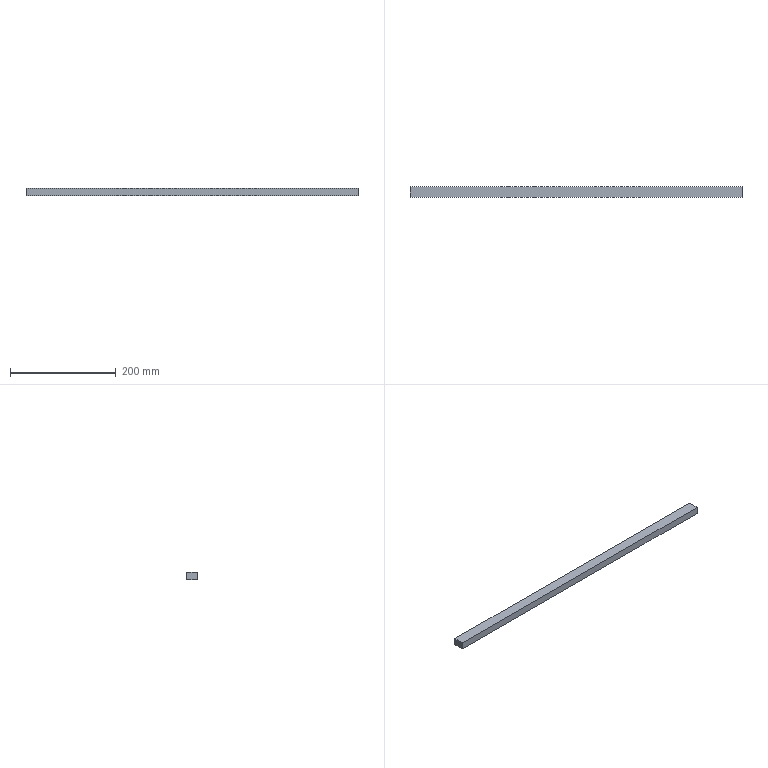Part | STEP file | Cylinder hanging plate | 1 solid | 6 faces | box 627.6 x 20 x 14 mm | volume 175728 mm3 | plane 6
STEP:
#1=CARTESIAN_POINT('',(0.,0.,0.));
#2=DIRECTION('',(0.,0.,1.));
#3=DIRECTION('',(1.,0.,0.));
#4=AXIS2_PLACEMENT_3D('',#1,#2,#3);
#5=CARTESIAN_POINT('',(313.8,-10.,0.));
#6=VERTEX_POINT('',#5);
#7=CARTESIAN_POINT('',(313.8,10.,0.));
#8=VERTEX_POINT('',#7);
#9=CARTESIAN_POINT('',(313.8,10.,0.));
#10=DIRECTION('',(0.,1.,0.));
#11=VECTOR('',#10,1.);
#12=LINE('',#9,#11);
#13=CARTESIAN_POINT('',(313.8,10.,14.));
#14=DIRECTION('',(-1.,0.,0.));
#15=DIRECTION('',(0.,0.,1.));
#16=AXIS2_PLACEMENT_3D('',#13,#14,#15);
#17=PLANE('',#16);
#18=CARTESIAN_POINT('',(-14.,0.));
#19=DIRECTION('',(0.,1.));
#20=VECTOR('',#19,1.);
#21=LINE('',#18,#20);
#22=(GEOMETRIC_REPRESENTATION_CONTEXT(2)PARAMETRIC_REPRESENTATION_CONTEXT()REPRESENTATION_CONTEXT('',''));
#23=DEFINITIONAL_REPRESENTATION('',(#21),#22);
#24=PCURVE('',#17,#23);
#25=CARTESIAN_POINT('',(313.8,-10.,0.));
#26=DIRECTION('',(0.,0.,1.));
#27=DIRECTION('',(1.,0.,0.));
#28=AXIS2_PLACEMENT_3D('',#25,#26,#27);
#29=PLANE('',#28);
#30=CARTESIAN_POINT('',(0.,20.));
#31=DIRECTION('',(0.,1.));
#32=VECTOR('',#31,1.);
#33=LINE('',#30,#32);
#34=(GEOMETRIC_REPRESENTATION_CONTEXT(2)PARAMETRIC_REPRESENTATION_CONTEXT()REPRESENTATION_CONTEXT('',''));
#35=DEFINITIONAL_REPRESENTATION('',(#33),#34);
#36=PCURVE('',#29,#35);
#37=SURFACE_CURVE('',#12,(#24,#36),.PCURVE_S1.);
#38=EDGE_CURVE('',#6,#8,#37,.T.);
#39=ORIENTED_EDGE('',*,*,#38,.T.);
#40=CARTESIAN_POINT('',(313.8,10.,14.));
#41=VERTEX_POINT('',#40);
#42=CARTESIAN_POINT('',(313.8,10.,14.));
#43=DIRECTION('',(0.,0.,-1.));
#44=VECTOR('',#43,1.);
#45=LINE('',#42,#44);
#46=CARTESIAN_POINT('',(0.,0.));
#47=DIRECTION('',(-1.,0.));
#48=VECTOR('',#47,1.);
#49=LINE('',#46,#48);
#50=(GEOMETRIC_REPRESENTATION_CONTEXT(2)PARAMETRIC_REPRESENTATION_CONTEXT()REPRESENTATION_CONTEXT('',''));
#51=DEFINITIONAL_REPRESENTATION('',(#49),#50);
#52=PCURVE('',#17,#51);
#53=CARTESIAN_POINT('',(-313.8,10.,14.));
#54=DIRECTION('',(0.,-1.,0.));
#55=DIRECTION('',(0.,0.,-1.));
#56=AXIS2_PLACEMENT_3D('',#53,#54,#55);
#57=PLANE('',#56);
#58=CARTESIAN_POINT('',(0.,627.6));
#59=DIRECTION('',(1.,0.));
#60=VECTOR('',#59,1.);
#61=LINE('',#58,#60);
#62=(GEOMETRIC_REPRESENTATION_CONTEXT(2)PARAMETRIC_REPRESENTATION_CONTEXT()REPRESENTATION_CONTEXT('',''));
#63=DEFINITIONAL_REPRESENTATION('',(#61),#62);
#64=PCURVE('',#57,#63);
#65=SURFACE_CURVE('',#45,(#52,#64),.PCURVE_S1.);
#66=EDGE_CURVE('',#41,#8,#65,.T.);
#67=ORIENTED_EDGE('',*,*,#66,.F.);
#68=CARTESIAN_POINT('',(313.8,-10.,14.));
#69=VERTEX_POINT('',#68);
#70=CARTESIAN_POINT('',(313.8,10.,14.));
#71=DIRECTION('',(0.,1.,0.));
#72=VECTOR('',#71,1.);
#73=LINE('',#70,#72);
#74=CARTESIAN_POINT('',(0.,0.));
#75=DIRECTION('',(0.,1.));
#76=VECTOR('',#75,1.);
#77=LINE('',#74,#76);
#78=(GEOMETRIC_REPRESENTATION_CONTEXT(2)PARAMETRIC_REPRESENTATION_CONTEXT()REPRESENTATION_CONTEXT('',''));
#79=DEFINITIONAL_REPRESENTATION('',(#77),#78);
#80=PCURVE('',#17,#79);
#81=CARTESIAN_POINT('',(313.8,-10.,14.));
#82=DIRECTION('',(0.,0.,1.));
#83=DIRECTION('',(1.,0.,0.));
#84=AXIS2_PLACEMENT_3D('',#81,#82,#83);
#85=PLANE('',#84);
#86=CARTESIAN_POINT('',(0.,20.));
#87=DIRECTION('',(0.,1.));
#88=VECTOR('',#87,1.);
#89=LINE('',#86,#88);
#90=(GEOMETRIC_REPRESENTATION_CONTEXT(2)PARAMETRIC_REPRESENTATION_CONTEXT()REPRESENTATION_CONTEXT('',''));
#91=DEFINITIONAL_REPRESENTATION('',(#89),#90);
#92=PCURVE('',#85,#91);
#93=SURFACE_CURVE('',#73,(#80,#92),.PCURVE_S1.);
#94=EDGE_CURVE('',#69,#41,#93,.T.);
#95=ORIENTED_EDGE('',*,*,#94,.F.);
#96=CARTESIAN_POINT('',(313.8,-10.,14.));
#97=DIRECTION('',(0.,0.,-1.));
#98=VECTOR('',#97,1.);
#99=LINE('',#96,#98);
#100=CARTESIAN_POINT('',(0.,-20.));
#101=DIRECTION('',(-1.,0.));
#102=VECTOR('',#101,1.);
#103=LINE('',#100,#102);
#104=(GEOMETRIC_REPRESENTATION_CONTEXT(2)PARAMETRIC_REPRESENTATION_CONTEXT()REPRESENTATION_CONTEXT('',''));
#105=DEFINITIONAL_REPRESENTATION('',(#103),#104);
#106=PCURVE('',#17,#105);
#107=CARTESIAN_POINT('',(-313.8,-10.,14.));
#108=DIRECTION('',(0.,1.,0.));
#109=DIRECTION('',(0.,0.,1.));
#110=AXIS2_PLACEMENT_3D('',#107,#108,#109);
#111=PLANE('',#110);
#112=CARTESIAN_POINT('',(0.,627.6));
#113=DIRECTION('',(-1.,0.));
#114=VECTOR('',#113,1.);
#115=LINE('',#112,#114);
#116=(GEOMETRIC_REPRESENTATION_CONTEXT(2)PARAMETRIC_REPRESENTATION_CONTEXT()REPRESENTATION_CONTEXT('',''));
#117=DEFINITIONAL_REPRESENTATION('',(#115),#116);
#118=PCURVE('',#111,#117);
#119=SURFACE_CURVE('',#99,(#106,#118),.PCURVE_S1.);
#120=EDGE_CURVE('',#69,#6,#119,.T.);
#121=ORIENTED_EDGE('',*,*,#120,.T.);
#122=EDGE_LOOP('',(#39,#67,#95,#121));
#123=FACE_BOUND('',#122,.T.);
#124=ADVANCED_FACE('',(#123),#17,.F.);
#125=CARTESIAN_POINT('',(-313.8,10.,0.));
#126=VERTEX_POINT('',#125);
#127=CARTESIAN_POINT('',(-313.8,10.,0.));
#128=DIRECTION('',(-1.,0.,0.));
#129=VECTOR('',#128,1.);
#130=LINE('',#127,#129);
#131=CARTESIAN_POINT('',(14.,0.));
#132=DIRECTION('',(0.,-1.));
#133=VECTOR('',#132,1.);
#134=LINE('',#131,#133);
#135=(GEOMETRIC_REPRESENTATION_CONTEXT(2)PARAMETRIC_REPRESENTATION_CONTEXT()REPRESENTATION_CONTEXT('',''));
#136=DEFINITIONAL_REPRESENTATION('',(#134),#135);
#137=PCURVE('',#57,#136);
#138=CARTESIAN_POINT('',(-627.6,20.));
#139=DIRECTION('',(-1.,0.));
#140=VECTOR('',#139,1.);
#141=LINE('',#138,#140);
#142=(GEOMETRIC_REPRESENTATION_CONTEXT(2)PARAMETRIC_REPRESENTATION_CONTEXT()REPRESENTATION_CONTEXT('',''));
#143=DEFINITIONAL_REPRESENTATION('',(#141),#142);
#144=PCURVE('',#29,#143);
#145=SURFACE_CURVE('',#130,(#137,#144),.PCURVE_S1.);
#146=EDGE_CURVE('',#8,#126,#145,.T.);
#147=ORIENTED_EDGE('',*,*,#146,.T.);
#148=CARTESIAN_POINT('',(-313.8,10.,14.));
#149=VERTEX_POINT('',#148);
#150=CARTESIAN_POINT('',(-313.8,10.,14.));
#151=DIRECTION('',(0.,0.,-1.));
#152=VECTOR('',#151,1.);
#153=LINE('',#150,#152);
#154=CARTESIAN_POINT('',(0.,0.));
#155=DIRECTION('',(1.,0.));
#156=VECTOR('',#155,1.);
#157=LINE('',#154,#156);
#158=(GEOMETRIC_REPRESENTATION_CONTEXT(2)PARAMETRIC_REPRESENTATION_CONTEXT()REPRESENTATION_CONTEXT('',''));
#159=DEFINITIONAL_REPRESENTATION('',(#157),#158);
#160=PCURVE('',#57,#159);
#161=CARTESIAN_POINT('',(-313.8,10.,14.));
#162=DIRECTION('',(1.,0.,0.));
#163=DIRECTION('',(0.,0.,-1.));
#164=AXIS2_PLACEMENT_3D('',#161,#162,#163);
#165=PLANE('',#164);
#166=CARTESIAN_POINT('',(0.,0.));
#167=DIRECTION('',(1.,0.));
#168=VECTOR('',#167,1.);
#169=LINE('',#166,#168);
#170=(GEOMETRIC_REPRESENTATION_CONTEXT(2)PARAMETRIC_REPRESENTATION_CONTEXT()REPRESENTATION_CONTEXT('',''));
#171=DEFINITIONAL_REPRESENTATION('',(#169),#170);
#172=PCURVE('',#165,#171);
#173=SURFACE_CURVE('',#153,(#160,#172),.PCURVE_S1.);
#174=EDGE_CURVE('',#149,#126,#173,.T.);
#175=ORIENTED_EDGE('',*,*,#174,.F.);
#176=CARTESIAN_POINT('',(-313.8,10.,14.));
#177=DIRECTION('',(-1.,0.,0.));
#178=VECTOR('',#177,1.);
#179=LINE('',#176,#178);
#180=CARTESIAN_POINT('',(0.,0.));
#181=DIRECTION('',(0.,-1.));
#182=VECTOR('',#181,1.);
#183=LINE('',#180,#182);
#184=(GEOMETRIC_REPRESENTATION_CONTEXT(2)PARAMETRIC_REPRESENTATION_CONTEXT()REPRESENTATION_CONTEXT('',''));
#185=DEFINITIONAL_REPRESENTATION('',(#183),#184);
#186=PCURVE('',#57,#185);
#187=CARTESIAN_POINT('',(-627.6,20.));
#188=DIRECTION('',(-1.,0.));
#189=VECTOR('',#188,1.);
#190=LINE('',#187,#189);
#191=(GEOMETRIC_REPRESENTATION_CONTEXT(2)PARAMETRIC_REPRESENTATION_CONTEXT()REPRESENTATION_CONTEXT('',''));
#192=DEFINITIONAL_REPRESENTATION('',(#190),#191);
#193=PCURVE('',#85,#192);
#194=SURFACE_CURVE('',#179,(#186,#193),.PCURVE_S1.);
#195=EDGE_CURVE('',#41,#149,#194,.T.);
#196=ORIENTED_EDGE('',*,*,#195,.F.);
#197=ORIENTED_EDGE('',*,*,#66,.T.);
#198=EDGE_LOOP('',(#147,#175,#196,#197));
#199=FACE_BOUND('',#198,.T.);
#200=ADVANCED_FACE('',(#199),#57,.F.);
#201=CARTESIAN_POINT('',(-313.8,-10.,0.));
#202=VERTEX_POINT('',#201);
#203=CARTESIAN_POINT('',(-313.8,10.,0.));
#204=DIRECTION('',(0.,-1.,0.));
#205=VECTOR('',#204,1.);
#206=LINE('',#203,#205);
#207=CARTESIAN_POINT('',(14.,0.));
#208=DIRECTION('',(0.,-1.));
#209=VECTOR('',#208,1.);
#210=LINE('',#207,#209);
#211=(GEOMETRIC_REPRESENTATION_CONTEXT(2)PARAMETRIC_REPRESENTATION_CONTEXT()REPRESENTATION_CONTEXT('',''));
#212=DEFINITIONAL_REPRESENTATION('',(#210),#211);
#213=PCURVE('',#165,#212);
#214=CARTESIAN_POINT('',(-627.6,20.));
#215=DIRECTION('',(0.,-1.));
#216=VECTOR('',#215,1.);
#217=LINE('',#214,#216);
#218=(GEOMETRIC_REPRESENTATION_CONTEXT(2)PARAMETRIC_REPRESENTATION_CONTEXT()REPRESENTATION_CONTEXT('',''));
#219=DEFINITIONAL_REPRESENTATION('',(#217),#218);
#220=PCURVE('',#29,#219);
#221=SURFACE_CURVE('',#206,(#213,#220),.PCURVE_S1.);
#222=EDGE_CURVE('',#126,#202,#221,.T.);
#223=ORIENTED_EDGE('',*,*,#222,.T.);
#224=CARTESIAN_POINT('',(-313.8,-10.,14.));
#225=VERTEX_POINT('',#224);
#226=CARTESIAN_POINT('',(-313.8,-10.,14.));
#227=DIRECTION('',(0.,0.,-1.));
#228=VECTOR('',#227,1.);
#229=LINE('',#226,#228);
#230=CARTESIAN_POINT('',(0.,-20.));
#231=DIRECTION('',(1.,0.));
#232=VECTOR('',#231,1.);
#233=LINE('',#230,#232);
#234=(GEOMETRIC_REPRESENTATION_CONTEXT(2)PARAMETRIC_REPRESENTATION_CONTEXT()REPRESENTATION_CONTEXT('',''));
#235=DEFINITIONAL_REPRESENTATION('',(#233),#234);
#236=PCURVE('',#165,#235);
#237=CARTESIAN_POINT('',(0.,0.));
#238=DIRECTION('',(-1.,0.));
#239=VECTOR('',#238,1.);
#240=LINE('',#237,#239);
#241=(GEOMETRIC_REPRESENTATION_CONTEXT(2)PARAMETRIC_REPRESENTATION_CONTEXT()REPRESENTATION_CONTEXT('',''));
#242=DEFINITIONAL_REPRESENTATION('',(#240),#241);
#243=PCURVE('',#111,#242);
#244=SURFACE_CURVE('',#229,(#236,#243),.PCURVE_S1.);
#245=EDGE_CURVE('',#225,#202,#244,.T.);
#246=ORIENTED_EDGE('',*,*,#245,.F.);
#247=CARTESIAN_POINT('',(-313.8,10.,14.));
#248=DIRECTION('',(0.,-1.,0.));
#249=VECTOR('',#248,1.);
#250=LINE('',#247,#249);
#251=CARTESIAN_POINT('',(0.,0.));
#252=DIRECTION('',(0.,-1.));
#253=VECTOR('',#252,1.);
#254=LINE('',#251,#253);
#255=(GEOMETRIC_REPRESENTATION_CONTEXT(2)PARAMETRIC_REPRESENTATION_CONTEXT()REPRESENTATION_CONTEXT('',''));
#256=DEFINITIONAL_REPRESENTATION('',(#254),#255);
#257=PCURVE('',#165,#256);
#258=CARTESIAN_POINT('',(-627.6,20.));
#259=DIRECTION('',(0.,-1.));
#260=VECTOR('',#259,1.);
#261=LINE('',#258,#260);
#262=(GEOMETRIC_REPRESENTATION_CONTEXT(2)PARAMETRIC_REPRESENTATION_CONTEXT()REPRESENTATION_CONTEXT('',''));
#263=DEFINITIONAL_REPRESENTATION('',(#261),#262);
#264=PCURVE('',#85,#263);
#265=SURFACE_CURVE('',#250,(#257,#264),.PCURVE_S1.);
#266=EDGE_CURVE('',#149,#225,#265,.T.);
#267=ORIENTED_EDGE('',*,*,#266,.F.);
#268=ORIENTED_EDGE('',*,*,#174,.T.);
#269=EDGE_LOOP('',(#223,#246,#267,#268));
#270=FACE_BOUND('',#269,.T.);
#271=ADVANCED_FACE('',(#270),#165,.F.);
#272=CARTESIAN_POINT('',(-313.8,-10.,0.));
#273=DIRECTION('',(1.,0.,0.));
#274=VECTOR('',#273,1.);
#275=LINE('',#272,#274);
#276=CARTESIAN_POINT('',(-14.,0.));
#277=DIRECTION('',(0.,1.));
#278=VECTOR('',#277,1.);
#279=LINE('',#276,#278);
#280=(GEOMETRIC_REPRESENTATION_CONTEXT(2)PARAMETRIC_REPRESENTATION_CONTEXT()REPRESENTATION_CONTEXT('',''));
#281=DEFINITIONAL_REPRESENTATION('',(#279),#280);
#282=PCURVE('',#111,#281);
#283=CARTESIAN_POINT('',(-627.6,0.));
#284=DIRECTION('',(1.,0.));
#285=VECTOR('',#284,1.);
#286=LINE('',#283,#285);
#287=(GEOMETRIC_REPRESENTATION_CONTEXT(2)PARAMETRIC_REPRESENTATION_CONTEXT()REPRESENTATION_CONTEXT('',''));
#288=DEFINITIONAL_REPRESENTATION('',(#286),#287);
#289=PCURVE('',#29,#288);
#290=SURFACE_CURVE('',#275,(#282,#289),.PCURVE_S1.);
#291=EDGE_CURVE('',#202,#6,#290,.T.);
#292=ORIENTED_EDGE('',*,*,#291,.T.);
#293=ORIENTED_EDGE('',*,*,#120,.F.);
#294=CARTESIAN_POINT('',(-313.8,-10.,14.));
#295=DIRECTION('',(1.,0.,0.));
#296=VECTOR('',#295,1.);
#297=LINE('',#294,#296);
#298=CARTESIAN_POINT('',(0.,0.));
#299=DIRECTION('',(0.,1.));
#300=VECTOR('',#299,1.);
#301=LINE('',#298,#300);
#302=(GEOMETRIC_REPRESENTATION_CONTEXT(2)PARAMETRIC_REPRESENTATION_CONTEXT()REPRESENTATION_CONTEXT('',''));
#303=DEFINITIONAL_REPRESENTATION('',(#301),#302);
#304=PCURVE('',#111,#303);
#305=CARTESIAN_POINT('',(-627.6,0.));
#306=DIRECTION('',(1.,0.));
#307=VECTOR('',#306,1.);
#308=LINE('',#305,#307);
#309=(GEOMETRIC_REPRESENTATION_CONTEXT(2)PARAMETRIC_REPRESENTATION_CONTEXT()REPRESENTATION_CONTEXT('',''));
#310=DEFINITIONAL_REPRESENTATION('',(#308),#309);
#311=PCURVE('',#85,#310);
#312=SURFACE_CURVE('',#297,(#304,#311),.PCURVE_S1.);
#313=EDGE_CURVE('',#225,#69,#312,.T.);
#314=ORIENTED_EDGE('',*,*,#313,.F.);
#315=ORIENTED_EDGE('',*,*,#245,.T.);
#316=EDGE_LOOP('',(#292,#293,#314,#315));
#317=FACE_BOUND('',#316,.T.);
#318=ADVANCED_FACE('',(#317),#111,.F.);
#319=ORIENTED_EDGE('',*,*,#94,.T.);
#320=ORIENTED_EDGE('',*,*,#195,.T.);
#321=ORIENTED_EDGE('',*,*,#266,.T.);
#322=ORIENTED_EDGE('',*,*,#313,.T.);
#323=EDGE_LOOP('',(#319,#320,#321,#322));
#324=FACE_BOUND('',#323,.T.);
#325=ADVANCED_FACE('',(#324),#85,.T.);
#326=ORIENTED_EDGE('',*,*,#38,.F.);
#327=ORIENTED_EDGE('',*,*,#291,.F.);
#328=ORIENTED_EDGE('',*,*,#222,.F.);
#329=ORIENTED_EDGE('',*,*,#146,.F.);
#330=EDGE_LOOP('',(#326,#327,#328,#329));
#331=FACE_BOUND('',#330,.T.);
#332=ADVANCED_FACE('',(#331),#29,.F.);
#333=CLOSED_SHELL('',(#124,#200,#271,#318,#325,#332));
#334=MANIFOLD_SOLID_BREP('',#333);
#335=(LENGTH_UNIT()NAMED_UNIT(*)SI_UNIT(.MILLI.,.METRE.));
#336=UNCERTAINTY_MEASURE_WITH_UNIT(LENGTH_MEASURE(0.0000001),#335,'','');
#337=(NAMED_UNIT(*)PLANE_ANGLE_UNIT()SI_UNIT($,.RADIAN.));
#338=(NAMED_UNIT(*)SI_UNIT($,.STERADIAN.)SOLID_ANGLE_UNIT());
#339=(GEOMETRIC_REPRESENTATION_CONTEXT(3)GLOBAL_UNCERTAINTY_ASSIGNED_CONTEXT((#336))GLOBAL_UNIT_ASSIGNED_CONTEXT((#335,#337,#338))REPRESENTATION_CONTEXT('',''));
#340=ADVANCED_BREP_SHAPE_REPRESENTATION('',(#4,#334),#339);